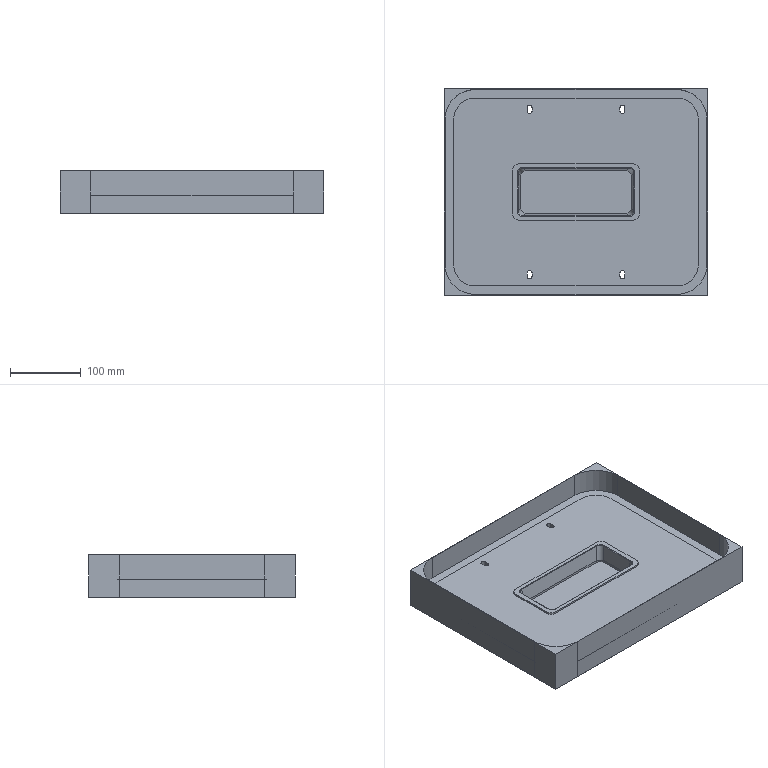NC program | NX | posted with a generic post | part box 371 x 291 x 60.5 mm
Lines 10591 to 11464 of 37416:
(CONTOUR_AREA , TOOL : R1.5)
N21174 M6
N21176 G53
N21178 G17 G0 G90 X-81.876 Y-39.38 S9000 M3 M8
N21180 G43 Z120.5 H0
N21182 Z31.3
N21184 G94 G1 Z28.3 F4500.
N21186 X-82.176 Y-39.321
N21188 X-82.462 Y-39.256
N21190 G2 X-85.472 Y-37.971 R8.221
N21192 G1 X-85.666 Y-37.853 Z28.298
N21194 X-85.775 Y-37.788 Z28.3
N21196 X-86.861 Y-36.859
N21198 X-87.633 Y-35.96
N21200 X-87.858 Y-35.66
N21202 X-87.873 Y-35.637
N21204 X-88.472 Y-34.658
N21206 X-88.565 Y-34.461
N21208 X-88.941 Y-33.562
N21210 X-89.074 Y-33.22
N21212 X-89.276 Y-32.367
N21214 X-89.374 Y-31.97
N21216 X-89.395 Y-31.764
N21218 X-89.486 Y-30.566
N21220 X-89.495 Y-29.967
N21222 Y30.264
N21224 X-89.486 Y30.554
N21226 Y30.566
N21228 X-89.396 Y31.75
N21230 X-89.374 Y31.97
N21232 X-89.205 Y32.663
N21234 X-89.074 Y33.22
N21236 X-88.941 Y33.56
N21238 X-88.566 Y34.458
N21240 X-88.474 Y34.656
N21242 X-87.874 Y35.636
N21244 X-87.858 Y35.66
N21246 X-87.635 Y35.958
N21248 X-86.861 Y36.859
N21250 X-85.775 Y37.788
N21252 X-84.575 Y38.51
N21254 X-83.375 Y39.013
N21256 X-83.075 Y39.102
N21258 X-82.176 Y39.319
N21260 X-81.876 Y39.38
N21262 X-80.676 Y39.483
N21264 X-80.376 Y39.496
N21266 X80.076
N21268 X80.376 Y39.492
N21270 X80.674 Y39.483
N21272 X81.855 Y39.382
N21274 X82.462 Y39.256
N21276 G2 X85.472 Y37.971 R8.221
N21278 G1 X85.666 Y37.853 Z28.298
N21280 X85.775 Y37.788 Z28.3
N21282 X86.861 Y36.859
N21284 X87.633 Y35.96
N21286 X87.873 Y35.637
N21288 X88.472 Y34.658
N21290 X88.565 Y34.461
N21292 X88.941 Y33.562
N21294 X89.074 Y33.22
N21296 X89.374 Y31.97
N21298 X89.395 Y31.764
N21300 X89.486 Y30.566
N21302 X89.494 Y30.266
N21304 X89.495 Y-29.967
N21306 X89.486 Y-30.554
N21308 X89.464 Y-30.855
N21310 X89.396 Y-31.75
N21312 X89.374 Y-31.97
N21314 X89.277 Y-32.364
N21316 X89.074 Y-33.22
N21318 X88.941 Y-33.56
N21320 X88.566 Y-34.458
N21322 X88.474 Y-34.656
N21324 X87.874 Y-35.637
N21326 X87.688 Y-35.886 Z28.299
N21328 X87.635 Y-35.958 Z28.3
N21330 X86.861 Y-36.859
N21332 X85.775 Y-37.788
N21334 X84.575 Y-38.51
N21336 X83.375 Y-39.013
N21338 X83.075 Y-39.102
N21340 X82.479 Y-39.251
N21342 X81.876 Y-39.38
N21344 X80.676 Y-39.483
N21346 X80.376 Y-39.492
N21348 X80.081 Y-39.496
N21350 X-80.372
N21352 X-80.674 Y-39.483
N21354 X-81.876 Y-39.38
N21356 X-81.84 Y-39.124
N21358 G2 X-86.722 Y-36.636 R8.88
N21360 X-88.876 Y-32.963 R8.803
N21362 G1 X-88.915 Y-32.804
N21364 X-89.02 Y-32.364
N21366 X-89.093 Y-32.064
N21368 X-89.139 Y-31.809
N21370 X-89.231 Y-30.566
N21372 X-89.245 Y-29.838
N21374 X-89.242 Y30.266
N21376 X-89.223 Y30.716
N21378 G2 X-83.375 Y38.74 R8.677
N21380 G1 X-83.244 Y38.788
N21382 G2 X-80.387 Y39.245 R9.754
N21384 G1 X80.366 Y39.246
N21386 G2 X86.722 Y36.636 R8.941
N21388 X88.875 Y32.963 R8.799
N21390 G1 X88.915 Y32.804
N21392 X88.949 Y32.663
N21394 X89.095 Y32.057
N21396 X89.136 Y31.807
N21398 X89.203 Y30.994
N21400 X89.238 Y30.43
N21402 X89.244 Y29.966
N21404 X89.243 Y-30.097
N21406 G2 X88.856 Y-33.034 R9.544
N21408 X88.174 Y-34.666 R7.729
N21410 G1 X87.874 Y-35.157
N21412 X87.747 Y-35.36
N21414 G2 X83.075 Y-38.837 R8.772
N21416 G1 X82.826 Y-38.906
N21418 X82.476 Y-38.994
N21420 X82.258 Y-39.043
N21422 G2 X80.387 Y-39.245 R9.523
N21424 G1 X-80.366
N21426 X-80.653 Y-39.233
N21428 X-81.755 Y-39.136
N21430 X-81.84 Y-39.124
N21432 X-81.798 Y-38.878
N21434 G2 X-88.981 Y-30.566 R8.474
N21436 G1 X-88.995 Y-29.887
N21438 X-88.99 Y30.349
N21440 G2 X-88.665 Y32.772 R9.062
N21442 X-82.788 Y38.657 R8.461
N21444 X-80.378 Y38.995 R9.822
N21446 G1 X-80.337
N21448 X80.375
N21450 G2 X85.596 Y37.279 R8.882
N21452 G1 X85.742 Y37.158
N21454 G2 X88.927 Y31.318 R8.336
N21456 G1 X88.986 Y30.478
N21458 X88.994 Y29.966
N21460 Y-30.046
N21462 G2 X88.665 Y-32.772 R9.424
N21464 X81.305 Y-38.927 R8.445
N21466 G1 X80.679 Y-38.981
N21468 X80.378 Y-38.995
N21470 X80.337
N21472 X-80.375
N21474 X-80.674 Y-38.981
N21476 X-81.528 Y-38.908
N21478 X-81.576 Y-38.903
N21480 X-81.798 Y-38.878
N21482 X-81.767 Y-38.629
N21484 G2 X-85.419 Y-37.102 R8.281
N21486 X-88.734 Y-30.526 R8.293
N21488 G1 X-88.74 Y-30.266
N21490 X-88.745 Y-29.937
N21492 X-88.743 Y30.297
N21494 G2 X-86.176 Y36.457 R8.436
N21496 X-80.076 Y38.745 R8.578
N21498 G1 X80.165
N21500 G2 X81.876 Y38.612 R13.516
N21502 X85.419 Y37.102 R8.783
N21504 X88.735 Y30.527 R8.297
N21506 G1 X88.744 Y30.236
N21508 X88.745 Y-29.966
N21510 G2 X88.297 Y-33.139 R9.253
N21512 G1 X88.094 Y-33.642
N21514 G2 X81.58 Y-38.653 R8.22
N21516 G1 X80.599 Y-38.733
N21518 X80.076 Y-38.745
N21520 X-80.165
N21522 G2 X-81.767 Y-38.629 R12.333
N21524 G1 X-81.733 Y-38.38
N21526 X-81.875 Y-38.36
N21528 G2 X-86.075 Y-36.212 R8.077
N21530 X-88.49 Y-30.285 R8.141
N21532 G1 X-88.495 Y-29.99
N21534 X-88.494 Y30.244
N21536 G2 X-86.016 Y36.259 R8.178
N21538 X-80.076 Y38.495 R8.262
N21540 G1 X80.214 Y38.494
N21542 G2 X84.275 Y37.522 R8.465
N21544 X88.482 Y30.576 R7.944
N21546 G1 X88.493 Y30.288
N21548 X88.495 Y-29.943
N21550 G2 X88.049 Y-33.088 R8.909
N21552 X80.548 Y-38.485 R8.037
N21554 G1 X80.076 Y-38.495
N21556 X-80.214 Y-38.494
N21558 X-80.676 Y-38.476
N21560 X-81.575 Y-38.401
N21562 X-81.733 Y-38.38
N21564 X-81.696 Y-38.13
N21566 G2 X-88.238 Y-30.33 R7.733
N21568 G1 X-88.243 Y-30.036
N21570 X-88.242 Y30.266
N21572 G2 X-88.119 Y31.819 R18.435
N21574 X-80.496 Y38.237 R7.781
N21576 G1 X-80.376 Y38.241
N21578 X-75.084 Y38.245
N21580 X80.263 Y38.244
N21582 G2 X84.894 Y36.859 R8.139
N21584 X88.242 Y30.266 R7.841
N21586 G1 X88.245 Y-29.896
N21588 G2 X88.119 Y-31.82 R16.142
N21590 X80.376 Y-38.241 R7.8
N21592 G1 X75.084 Y-38.245
N21594 X-80.263 Y-38.244
N21596 X-80.676 Y-38.226
N21598 X-81.576 Y-38.146
N21600 X-81.655 Y-38.136
N21602 X-81.696 Y-38.13
N21604 X-81.662 Y-37.881
N21606 G2 X-84.896 Y-36.559 R7.717
N21608 X-87.978 Y-30.566 R7.545
N21610 G1 X-87.993 Y-30.085
N21612 X-87.991 Y30.266
N21614 G2 X-84.875 Y36.557 R7.51
N21616 X-80.376 Y37.991 R7.778
N21618 G1 X80.312 Y37.993
N21620 G2 X84.896 Y36.559 R7.847
N21622 X87.979 Y30.566 R7.549
N21624 G1 X87.993 Y30.085
N21626 X87.992 Y-30.148
N21628 G2 X87.689 Y-32.549 R8.536
N21630 X80.444 Y-37.99 R7.546
N21632 G1 X80.376 Y-37.991
N21634 X-80.312 Y-37.993
N21636 X-80.676 Y-37.976
N21638 X-81.429 Y-37.91
N21640 X-81.576 Y-37.893
N21642 X-81.662 Y-37.881
N21644 X-81.623 Y-37.633
N21646 G2 X-87.719 Y-30.71 R7.214
N21648 G1 X-87.739 Y-30.266
N21650 X-87.745 Y-29.667
N21652 X-87.74 Y30.266
N21654 G2 X-87.444 Y32.494 R8.225
N21656 X-80.71 Y37.723 R7.267
N21658 G1 X-80.391 Y37.743
N21660 X80.362 Y37.744
N21662 G2 X85.798 Y35.41 R7.403
N21664 X87.728 Y30.566 R7.254
N21666 G1 X87.743 Y30.135
N21668 X87.742 Y-30.098
N21670 G2 X87.293 Y-32.961 R8.388
N21672 X80.71 Y-37.723 R7.266
N21674 G1 X80.391 Y-37.743
N21676 X-80.362 Y-37.744
N21678 X-80.647 Y-37.728
N21680 X-81.472 Y-37.654
N21682 X-81.576 Y-37.64
N21684 X-81.623 Y-37.633
N21686 X-81.576 Y-37.388
N21688 G2 X-87.444 Y-31.035 R6.93
N21690 G1 X-87.482 Y-30.474
N21692 X-87.495 Y-29.887
N21694 X-87.491 Y30.266
N21696 G2 X-87.2 Y32.438 R8.021
N21698 X-80.678 Y37.475 R7.013
N21700 G1 X-80.378 Y37.493
N21702 X80.375
N21704 G2 X82.576 Y37.158 R8.238
N21706 X87.465 Y30.756 R6.936
N21708 G1 X87.49 Y30.266
N21710 X87.493 Y-30.047
N21712 G2 X87.2 Y-32.437 R8.292
N21714 X80.678 Y-37.475 R7.014
N21716 G1 X80.378 Y-37.493
N21718 X-80.375
N21720 G2 X-81.576 Y-37.388 R20.153
N21722 G1 X-81.558 Y-37.14
N21724 G2 X-87.231 Y-30.522 R6.727
N21726 G1 X-87.24 Y-30.232
N21728 X-87.245 Y-29.937
N21730 X-87.241 Y30.299
N21732 G2 X-86.958 Y32.38 R7.788
N21734 X-80.376 Y37.239 R6.804
N21736 G1 X-80.292 Y37.242
N21738 X80.162 Y37.244
N21740 G2 X83.405 Y36.559 R7.492
N21742 X87.231 Y30.522 R6.711
N21744 G1 X87.242 Y30.266
N21746 Y30.234
N21748 X87.244 Y-29.997
N21750 G2 X86.974 Y-32.319 R8.104
N21752 X80.376 Y-37.239 R6.81
N21754 G1 X80.292 Y-37.242
N21756 X-80.162 Y-37.244
N21758 G2 X-81.558 Y-37.14 R13.174
N21760 G1 X-81.526 Y-36.89
N21762 G2 X-85.175 Y-34.983 R6.642
N21764 X-86.989 Y-30.283 R6.6
N21766 G1 X-86.994 Y-29.989
N21768 X-86.993 Y30.245
N21770 G2 X-86.712 Y32.326 R8.362
N21772 X-80.554 Y36.981 R6.552
N21774 G1 X-80.076 Y36.994
N21776 X80.211 Y36.993
N21778 G2 X83.451 Y36.259 R7.021
N21780 X86.992 Y30.287 R6.567
N21782 G1 X86.995 Y-29.944
N21784 G2 X86.891 Y-31.548 R15.293
N21786 X80.554 Y-36.981 R6.538
N21788 G1 X80.076 Y-36.994
N21790 X-80.211 Y-36.993
N21792 X-80.676 Y-36.971
N21794 X-81.332 Y-36.914
N21796 X-81.526 Y-36.89
N21798 X-81.491 Y-36.639
N21800 G2 X-86.724 Y-30.618 R6.204
N21802 G1 X-86.743 Y-30.035
N21804 X-86.74 Y30.266
N21806 G2 X-82.476 Y36.39 R6.285
N21808 X-80.376 Y36.738 R6.535
N21810 G1 X-79.891 Y36.744
N21812 X80.26 Y36.742
N21814 G2 X84.323 Y35.409 R6.542
N21816 X86.724 Y30.618 R6.252
N21818 G1 X86.738 Y30.33
N21820 X86.74 Y30.266
N21822 X86.744 Y-29.897
N21824 G2 X86.519 Y-32.064 R7.88
N21826 X80.976 Y-36.697 R6.252
N21828 G1 X80.376 Y-36.738
N21830 X79.891 Y-36.744
N21832 X-80.26 Y-36.742
N21834 X-80.676 Y-36.721
N21836 X-81.373 Y-36.655
N21838 X-81.491 Y-36.639
N21840 X-81.45 Y-36.39
N21842 G2 X-86.475 Y-30.566 R5.969
N21844 G1 X-86.493 Y-29.966
N21846 X-86.492 Y30.149
N21848 G2 X-86.324 Y31.815 R8.539
N21850 X-80.976 Y36.446 R6.002
N21852 G1 X-80.376 Y36.489
N21854 X-80.142 Y36.493
N21856 X-79.841 Y36.494
N21858 X80.076 Y36.495
N21860 G2 X82.379 Y36.163 R7.225
N21862 X86.475 Y30.566 R5.962
N21864 G1 X86.492 Y30.084
N21866 X86.493 Y-29.966
N21868 G2 X86.323 Y-31.816 R8.65
N21870 X80.976 Y-36.446 R6.
N21872 G1 X80.376 Y-36.489
N21874 X80.142 Y-36.493
N21876 X79.841 Y-36.494
N21878 X-80.076 Y-36.495
N21880 G2 X-81.45 Y-36.39 R9.833
N21882 G1 X-81.414 Y-36.142
N21884 G2 X-86.224 Y-30.566 R5.692
N21886 G1 X-86.243 Y-29.966
N21888 X-86.242 Y30.099
N21890 G2 X-86.08 Y31.761 R8.098
N21892 X-81.047 Y36.189 R5.758
N21894 G1 X-80.376 Y36.24
N21896 X80.063 Y36.246
N21898 G2 X83.038 Y35.622 R6.562
N21900 X86.224 Y30.566 R5.735
N21902 G1 X86.241 Y30.133
N21904 Y-30.099
N21906 G2 X86.079 Y-31.759 R7.93
N21908 X81.047 Y-36.189 R5.755
N21910 G1 X80.376 Y-36.24
N21912 X-80.063 Y-36.246
N21914 G2 X-81.414 Y-36.142 R11.267
N21916 G1 X-81.374 Y-35.895
N21918 G2 X-85.973 Y-30.566 R5.472
N21920 G1 X-85.99 Y-30.181
N21922 X-85.995 Y-28.744
N21924 X-85.989 Y30.266
N21926 G2 X-85.635 Y32.364 R5.858
N21928 X-80.678 Y35.97 R5.547
N21930 G1 X-80.378 Y35.991
N21932 X80.075 Y35.995
N21934 G2 X83.075 Y35.322 R6.189
N21936 X85.98 Y30.471 R5.496
N21938 G1 X85.988 Y30.266
N21940 X85.991 Y30.182
N21942 X85.992 Y-30.049
N21944 G2 X85.731 Y-32.108 R7.171
N21946 X80.678 Y-35.97 R5.542
N21948 G1 X80.378 Y-35.991
N21950 X-80.075 Y-35.995
N21952 G2 X-81.374 Y-35.895 R10.8
N21954 G1 X-81.33 Y-35.65
N21956 G2 X-85.727 Y-30.518 R5.238
N21958 G1 X-85.739 Y-30.23
N21960 X-85.744 Y-29.936
N21962 X-85.739 Y30.302
N21964 G2 X-85.175 Y32.802 R5.596
N21966 X-80.296 Y35.74 R5.36
N21968 G1 X80.159 Y35.743
N21970 G2 X83.029 Y35.061 R5.767
N21972 X85.727 Y30.518 R5.223
N21974 G1 X85.74 Y30.266
N21976 X85.741 Y30.232
N21978 X85.743 Y-29.998
N21980 G2 X85.296 Y-32.542 R6.203
N21982 X80.296 Y-35.74 R5.34
N21984 G1 X-80.16 Y-35.743
N21986 G2 X-81.33 Y-35.65 R10.7
N21988 G1 X-81.276 Y-35.406
N21990 G2 X-85.474 Y-30.566 R4.977
N21992 G1 X-85.488 Y-30.282
N21994 X-85.494 Y-29.988
N21996 X-85.492 Y30.247
N21998 G2 X-85.043 Y32.495 R5.441
N22000 X-80.561 Y35.476 R5.077
N22002 G1 X-80.076 Y35.493
N22004 X80.076 Y35.494
N22006 G2 X82.256 Y35.141 R5.591
N22008 X85.474 Y30.566 R4.961
N22010 G1 X85.49 Y30.284
N22012 X85.494 Y-29.945
N22014 G2 X85.346 Y-31.594 R8.901
N22016 X80.676 Y-35.467 R5.035
N22018 G1 X80.246 Y-35.491
N22020 X-80.076 Y-35.494
N22022 X-80.495 Y-35.479
N22024 X-81.048 Y-35.432
N22026 X-81.276 Y-35.406
N22028 X-81.243 Y-35.154
N22030 G2 X-85.22 Y-30.614 R4.701
N22032 G1 X-85.235 Y-30.326
N22034 X-85.244 Y-29.736
N22036 X-85.238 Y30.266
N22038 G2 X-85.104 Y31.536 R8.022
N22040 X-80.676 Y35.216 R4.796
N22042 G1 X-80.195 Y35.241
N22044 X80.076 Y35.243
N22046 G2 X82.271 Y34.865 R5.459
N22048 X85.22 Y30.614 R4.704
N22050 G1 X85.237 Y30.328
N22052 X85.243 Y28.816
N22054 Y-29.966
N22056 G2 X85.102 Y-31.537 R8.119
N22058 X80.676 Y-35.216 R4.792
N22060 G1 X80.195 Y-35.241
N22062 X-80.076 Y-35.243
N22064 X-80.541 Y-35.225
N22066 X-81.09 Y-35.174
N22068 X-81.243 Y-35.154
N22070 X-81.203 Y-34.904
N22072 G2 X-84.943 Y-30.934 R4.436
N22074 G1 X-84.981 Y-30.372
N22076 X-84.994 Y-29.786
N22078 X-84.99 Y30.151
N22080 G2 X-84.741 Y31.898 R5.317
N22082 X-80.376 Y34.985 R4.578
N22084 G1 X-79.843 Y34.994
N22086 X80.076
N22088 G2 X82.481 Y34.5 R5.375
N22090 X84.943 Y30.934 R4.427
N22092 G1 X84.982 Y30.373
N22094 X84.992 Y29.784
N22096 Y-29.966
N22098 X84.977 Y-30.463
N22100 G2 X80.376 Y-34.985 R4.558
N22102 G1 X79.843 Y-34.994
N22104 X-80.076
N22106 X-80.304 Y-34.989
N22108 X-80.376 Y-34.985
N22110 X-80.863 Y-34.947
N22112 X-81.203 Y-34.904
N22114 X-81.172 Y-34.657
N22116 G2 X-84.696 Y-30.865 R4.176
N22118 G1 X-84.728 Y-30.419
N22120 X-84.744 Y-29.835
N22122 X-84.74 Y30.101
N22124 G2 X-84.402 Y32.064 R4.904
N22126 X-80.376 Y34.736 R4.36
N22128 G1 X-80.076 Y34.744
N22130 X-76.494
N22132 X80.06 Y34.745
N22134 G2 X82.476 Y34.221 R5.07
N22136 X84.696 Y30.865 R4.148
N22138 G1 X84.729 Y30.42
N22140 X84.742 Y29.966
N22142 Y-29.966
N22144 G2 X84.494 Y-31.845 R6.157
N22146 X80.376 Y-34.736 R4.377
N22148 G1 X80.076 Y-34.744
N22150 X76.494
N22152 X-80.06 Y-34.745
N22154 G2 X-81.172 Y-34.657 R7.776
N22156 G1 X-81.134 Y-34.409
N22158 G2 X-84.444 Y-30.865 R3.913
N22160 G1 X-84.475 Y-30.466
N22162 X-84.493 Y-29.966
N22164 X-84.491 Y30.051
N22166 G2 X-84.258 Y31.764 R5.752
N22168 X-80.376 Y34.487 R4.117
N22170 G1 X-80.078 Y34.494
N22172 X-76.779
N22174 X-74.68 Y34.495 Z28.282
N22176 X75.278 Y34.496 Z28.284
N22178 X76.741 Y34.495 Z28.3
N22180 X80.074
N22182 G2 X82.176 Y34.086 R4.762
N22184 X84.476 Y30.467 R3.972
N22186 G1 X84.486 Y30.266
N22188 X84.489 Y30.18
N22190 X84.491 Y-30.05
N22192 G2 X84.259 Y-31.764 R5.341
N22194 X80.376 Y-34.487 R4.118
N22196 G1 X80.078 Y-34.494
N22198 X76.779
N22200 X74.68 Y-34.495 Z28.282
N22202 X-75.278 Y-34.496 Z28.284
N22204 X-76.741 Y-34.495 Z28.3
N22206 X-80.074
N22208 G2 X-81.134 Y-34.409 R8.021
N22210 G1 X-81.114 Y-34.162
N22212 G2 X-84.2 Y-30.791 R3.703
N22214 G1 X-84.236 Y-30.266
N22216 X-84.244 Y-29.667
N22218 X-84.241 Y30.
N22220 G2 X-83.99 Y31.762 R5.216
N22222 X-80.376 Y34.233 R3.857
N22224 G1 X-79.776 Y34.244
N22226 X-77.212 Z28.297
N22228 X-75.878 Y34.247 Z28.255
N22230 X-74.678 Y34.248 Z28.242
N22232 X75.278 Y34.249 Z28.245
N22234 X76.477 Y34.247 Z28.271
N22236 X77.21 Y34.245 Z28.297
N22238 X79.86 Z28.3
N22240 G2 X81.576 Y34.048 R5.447
N22242 X84.2 Y30.791 R3.648
N22244 G1 X84.239 Y30.23
N22246 X84.243 Y-29.998
N22248 G2 X83.99 Y-31.762 R5.276
N22250 X80.376 Y-34.233 R3.857
N22252 G1 X79.776 Y-34.244
N22254 X77.212 Z28.297
N22256 X75.878 Y-34.247 Z28.255
N22258 X74.678 Y-34.248 Z28.242
N22260 X-75.278 Y-34.249 Z28.245
N22262 X-76.477 Y-34.247 Z28.271
N22264 X-77.21 Y-34.245 Z28.297
N22266 X-79.86 Z28.3
N22268 G2 X-81.114 Y-34.162 R8.529
N22270 G1 X-81.068 Y-33.913
N22272 G2 X-83.975 Y-30.476 R3.466
N22274 G1 X-83.986 Y-30.279
N22276 X-83.994 Y-29.987
N22278 X-83.989 Y30.25
N22280 G2 X-82.551 Y33.263 R3.632
N22282 X-80.376 Y33.982 R3.663
N22284 G1 X-79.945 Y33.993
N22286 X-79.776 Y33.994
N22288 X-79.177
N22290 X-78.145
N22292 X-77.977 Z28.294
N22294 X-77.845
N22296 X-75.878 Y34.001 Z28.208
N22298 X-75.136 Y34.004 Z28.191
N22300 X-73.511 Z28.186
N22302 X74.978 Y34.005 Z28.188
N22304 X75.737 Y34.003 Z28.205
N22306 X76.777 Y33.999 Z28.245
N22308 X77.543 Y33.996 Z28.282
N22310 X78.144 Y33.995 Z28.3
N22312 X78.443
N22314 X79.477
N22316 G2 X81.325 Y33.862 R7.867
N22318 X83.946 Y30.836 R3.438
N22320 G1 X83.987 Y30.281
N22322 X83.992 Y29.986
N22324 X83.994 Y-29.945
N22326 G2 X83.675 Y-31.856 R4.506
N22328 X80.376 Y-33.982 R3.596
N22330 G1 X79.945 Y-33.993
N22332 X79.776 Y-33.994
N22334 X79.177
N22336 X78.145
N22338 X77.977 Z28.294
N22340 X77.845
N22342 X75.878 Y-34.001 Z28.208
N22344 X75.136 Y-34.004 Z28.191
N22346 X73.511 Z28.186
N22348 X-74.978 Y-34.005 Z28.188
N22350 X-75.737 Y-34.003 Z28.205
N22352 X-76.777 Y-33.999 Z28.245
N22354 X-77.543 Y-33.996 Z28.282
N22356 X-78.144 Y-33.995 Z28.3
N22358 X-78.443
N22360 X-79.477
N22362 X-80.204 Y-33.989
N22364 X-80.676 Y-33.959
N22366 X-81.033 Y-33.919
N22368 X-81.068 Y-33.913
N22370 X-81.028 Y-33.662
N22372 G2 X-83.715 Y-30.61 R3.18
N22374 G1 X-83.733 Y-30.325
N22376 X-83.744 Y-29.735
N22378 X-83.738 Y30.203
N22380 G2 X-83.492 Y31.647 R3.994
N22382 X-80.376 Y33.731 R3.332
N22384 G1 X-79.895 Y33.743
N22386 X-79.295 Y33.744
N22388 X-78.513 Z28.299
N22390 X-77.793 Y33.746 Z28.262
N22392 X-76.888 Y33.751 Z28.205
N22394 X-76.777 Y33.753 Z28.193
N22396 X-76.283 Y33.757 Z28.163
N22398 X-76.178 Y33.76 Z28.152
N22400 X-75.578 Y33.765 Z28.121
N22402 X-74.678 Y33.769 Z28.103
N22404 X74.978 Z28.107
N22406 X75.578 Y33.766 Z28.121
N22408 X76.178 Y33.761 Z28.153
N22410 X76.585 Y33.755 Z28.185
N22412 X76.777 Y33.754 Z28.194
N22414 X76.887 Y33.752 Z28.205
N22416 X78.093 Y33.746 Z28.281
N22418 X78.277 Z28.287
N22420 X78.511 Y33.745 Z28.299
N22422 X78.877 Z28.3
N22424 X79.659
N22426 G2 X81.318 Y33.604 R6.883
N22428 X83.715 Y30.61 R3.193
N22430 G1 X83.734 Y30.326
N22432 X83.741 Y30.032
N22434 X83.742 Y29.734
N22436 Y-29.966
N22438 X83.722 Y-30.519
N22440 G2 X80.376 Y-33.731 R3.322
N22442 G1 X79.895 Y-33.743
N22444 X79.295 Y-33.744
N22446 X78.513 Z28.299
N22448 X77.793 Y-33.746 Z28.262
N22450 X76.888 Y-33.751 Z28.205
N22452 X76.777 Y-33.753 Z28.193
N22454 X76.283 Y-33.757 Z28.163
N22456 X76.178 Y-33.76 Z28.152
N22458 X75.578 Y-33.765 Z28.121
N22460 X74.678 Y-33.769 Z28.103
N22462 X-74.978 Z28.107
N22464 X-75.578 Y-33.766 Z28.121
N22466 X-76.178 Y-33.761 Z28.153
N22468 X-76.585 Y-33.755 Z28.185
N22470 X-76.777 Y-33.754 Z28.194
N22472 X-76.887 Y-33.752 Z28.205
N22474 X-78.093 Y-33.746 Z28.281
N22476 X-78.277 Z28.287
N22478 X-78.511 Y-33.745 Z28.299
N22480 X-78.877 Z28.3
N22482 X-79.659
N22484 X-80.251 Y-33.737
N22486 X-80.676 Y-33.707
N22488 X-81.028 Y-33.662
N22490 X-80.976 Y-33.416
N22492 G2 X-83.438 Y-30.865 R2.923
N22494 G1 X-83.478 Y-30.369
N22496 X-83.492 Y-29.966
N22498 X-83.488 Y30.153
N22500 G2 X-83.394 Y31.154 R6.014
N22502 X-80.376 Y33.481 R3.105
N22504 G1 X-80.148 Y33.491
N22506 X-80.076 Y33.492
N22508 X-79.845 Y33.494
N22510 X-79.245
N22512 X-78.877 Z28.294
N22514 X-78.645 Z28.286
N22516 X-78.577 Y33.495 Z28.28
N22518 X-77.499 Y33.501 Z28.199
N22520 X-76.477 Y33.52 Z28.09
N22522 X-76.213 Y33.527 Z28.062
N22524 X-76.178 Y33.528 Z28.058
N22526 X-75.578 Y33.539 Z28.015
N22528 X-75.278 Y33.542 Z28.003
N22530 X-74.997 Y33.543 Z27.996
N22532 X-74.678 Y33.545 Z27.991
N22534 X74.662 Y33.546
N22536 X74.978 Y33.545 Z27.996
N22538 X75.278 Y33.543 Z28.003
N22540 X75.578 Y33.54 Z28.015
N22542 X76.212 Y33.528 Z28.063
N22544 X77.077 Y33.51 Z28.153
N22546 X77.497 Y33.502 Z28.199
N22548 X78.644 Y33.495 Z28.286
N22550 X78.877 Z28.294
N22552 X78.944 Z28.299
N22554 X79.709 Z28.3
N22556 G2 X81.57 Y33.257 R5.443
N22558 X83.479 Y30.369 R2.994
N22560 G1 X83.491 Y29.966
N22562 X83.492 Y-29.966
N22564 X83.473 Y-30.468
N22566 G2 X80.376 Y-33.481 R3.074
N22568 G1 X80.148 Y-33.491
N22570 X80.076 Y-33.492
N22572 X79.845 Y-33.494
N22574 X79.245
N22576 X78.877 Z28.294
N22578 X78.645 Z28.286
N22580 X78.577 Y-33.495 Z28.28
N22582 X77.499 Y-33.501 Z28.199
N22584 X76.477 Y-33.52 Z28.09
N22586 X76.213 Y-33.526 Z28.062
N22588 X76.169 Y-33.528 Z28.057
N22590 X75.9 Y-33.532 Z28.038
N22592 X75.578 Y-33.539 Z28.015
N22594 X75.278 Y-33.542 Z28.003
N22596 X74.997 Y-33.543 Z27.996
N22598 X74.678 Y-33.545 Z27.991
N22600 X-74.662 Y-33.546
N22602 X-74.978 Y-33.545 Z27.996
N22604 X-75.278 Y-33.543 Z28.003
N22606 X-75.578 Y-33.54 Z28.015
N22608 X-76.212 Y-33.528 Z28.063
N22610 X-77.077 Y-33.51 Z28.153
N22612 X-77.497 Y-33.502 Z28.199
N22614 X-78.644 Y-33.495 Z28.286
N22616 X-78.877 Z28.294
N22618 X-78.944 Z28.299
N22620 X-79.709 Z28.3
N22622 G2 X-80.976 Y-33.416 R7.385
N22624 G1 X-80.932 Y-33.169
N22626 G2 X-83.213 Y-30.566 R2.691
N22628 G1 X-83.238 Y-30.129
N22630 X-83.244 Y-29.667
N22632 X-83.239 Y30.103
N22634 G2 X-83.023 Y31.465 R3.669
N22636 X-80.376 Y33.232 R2.879
N22638 G1 X-80.096 Y33.243
N22640 X-79.795 Y33.244
N22642 X-79.477
N22644 X-79.214 Z28.296
N22646 X-78.277 Y33.249 Z28.219
N22648 X-77.988 Y33.252 Z28.191
N22650 X-77.977 Z28.189
N22652 X-77.377 Y33.266 Z28.104
N22654 X-76.75 Y33.29 Z28.006
N22656 X-76.131 Y33.309 Z27.934
N22658 X-75.518 Y33.322 Z27.888
N22660 X-75.283 Y33.326 Z27.876
N22662 X-74.982 Y33.328 Z27.868
N22664 X-74.682 Y33.33 Z27.863
N22666 X74.674 Y33.331 Z27.864
N22668 X75.278 Y33.327 Z27.877
N22670 X75.513 Y33.323 Z27.888
N22672 X75.578 Z27.891
N22674 X76.178 Y33.31 Z27.938
N22676 X76.777 Y33.291 Z28.009
N22678 X77.681 Y33.259 Z28.151
N22680 X77.977 Y33.253 Z28.19
N22682 X77.987 Z28.191
N22684 X78.893 Y33.246 Z28.273
N22686 X79.212 Y33.245 Z28.296
N22688 X79.477 Z28.3
N22690 X79.776
N22692 X80.076 Y33.239
N22694 G2 X82.176 Y32.634 R3.4
N22696 X83.214 Y30.566 R2.743
N22698 G1 X83.238 Y30.129
N22700 X83.242 Y26.913
N22702 X83.241 Y-29.966
N22704 G2 X82.987 Y-31.553 R3.803
N22706 X80.376 Y-33.232 R2.888
N22708 G1 X80.096 Y-33.243
N22710 X79.795 Y-33.244
N22712 X79.477
N22714 X79.214 Z28.296
N22716 X78.277 Y-33.249 Z28.219
N22718 X77.988 Y-33.252 Z28.191
N22720 X77.977 Z28.189
N22722 X77.377 Y-33.266 Z28.104
N22724 X76.75 Y-33.29 Z28.006
N22726 X76.116 Y-33.311 Z27.93
N22728 X75.518 Y-33.322 Z27.888
N22730 X75.283 Y-33.326 Z27.876
N22732 X74.982 Y-33.328 Z27.868
N22734 X74.682 Y-33.33 Z27.863
N22736 X-74.674 Y-33.331 Z27.864
N22738 X-75.278 Y-33.327 Z27.877
N22740 X-75.513 Y-33.323 Z27.888
N22742 X-75.578 Z27.891
N22744 X-76.178 Y-33.31 Z27.938
N22746 X-76.777 Y-33.291 Z28.009
N22748 X-77.681 Y-33.259 Z28.151
N22750 X-77.977 Y-33.253 Z28.19
N22752 X-77.987 Z28.191
N22754 X-79.177 Y-33.245 Z28.293
N22756 X-79.776 Z28.3
N22758 X-80.076 Y-33.239
N22760 G2 X-80.932 Y-33.169 R5.319
N22762 G1 X-80.896 Y-32.922
N22764 G2 X-82.962 Y-30.566 R2.441
N22766 G1 X-82.971 Y-30.461
N22768 X-82.992 Y-29.966
N22770 X-82.989 Y30.052
N22772 G2 X-82.731 Y31.51 R3.32
N22774 X-80.379 Y32.982 R2.64
N22776 G1 X-80.078 Y32.993
N22778 X-79.715 Y32.994
N22780 X-79.477 Z28.291
N22782 X-78.539 Y33.001 Z28.202
N22784 X-78.279 Y33.006 Z28.162
N22786 X-78.234 Z28.157
N22788 X-77.979 Y33.016 Z28.108
N22790 X-77.923 Y33.017 Z28.101
N22792 X-77.293 Y33.047 Z27.977
N22794 X-76.98 Y33.06 Z27.925
N22796 X-76.777 Y33.071 Z27.889
N22798 X-76.178 Y33.099 Z27.803
N22800 X-76.039 Y33.102 Z27.791
N22802 X-75.878 Y33.111 Z27.77
N22804 X-75.727 Y33.113 Z27.759
N22806 X-75.578 Y33.121 Z27.743
N22808 X-75.418 Y33.122 Z27.736
N22810 X-75.278 Y33.128 Z27.725
N22812 X-74.508 Y33.133 Z27.709
N22814 X74.808 Y33.132 Z27.714
N22816 X75.278 Y33.129 Z27.726
N22818 X75.417 Y33.123 Z27.736
N22820 X75.578 Y33.122 Z27.744
N22822 X75.726 Y33.114 Z27.76
N22824 X75.878 Y33.112 Z27.771
N22826 X76.178 Y33.095 Z27.81
N22828 X76.219 Y33.092 Z27.817
N22830 X76.477 Y33.085 Z27.846
N22832 X76.665 Y33.075 Z27.876
N22834 X76.777 Y33.072 Z27.89
N22836 X77.377 Y33.045 Z27.991
N22838 X77.921 Y33.018 Z28.101
N22840 X78.277 Y33.007 Z28.162
N22842 X78.536 Y33.002 Z28.202
N22844 X78.577 Y33.001 Z28.206
N22846 X79.477 Y32.995 Z28.291
N22848 X79.713 Z28.3
N22850 X80.043 Y32.994
N22852 X80.076
N22854 G2 X81.972 Y32.473 R3.172
N22856 X82.971 Y30.461 R2.52
N22858 G1 X82.983 Y30.266
N22860 X82.987 Y30.177
N22862 X82.992 Y29.667
N22864 X82.99 Y-30.051
N22866 G2 X82.731 Y-31.509 R3.357
N22868 X80.379 Y-32.982 R2.64
N22870 G1 X80.078 Y-32.993
N22872 X79.715 Y-32.994
N22874 X79.477 Z28.291
N22876 X78.539 Y-33.001 Z28.202
N22878 X78.279 Y-33.006 Z28.162
N22880 X78.234 Z28.157
N22882 X77.979 Y-33.016 Z28.108
N22884 X77.923 Y-33.017 Z28.101
N22886 X77.293 Y-33.047 Z27.977
N22888 X76.98 Y-33.06 Z27.925
N22890 X76.777 Y-33.071 Z27.889
N22892 X75.987 Y-33.108 Z27.778
N22894 X75.727 Y-33.113 Z27.759
N22896 X75.578 Y-33.121 Z27.743
N22898 X75.418 Y-33.122 Z27.736
N22900 X75.278 Y-33.128 Z27.725
N22902 X74.678 Y-33.133 Z27.71
N22904 X-74.808 Y-33.132 Z27.714
N22906 X-75.278 Y-33.129 Z27.726
N22908 X-75.417 Y-33.123 Z27.736
N22910 X-75.578 Y-33.122 Z27.744
N22912 X-75.726 Y-33.114 Z27.76
N22914 X-75.878 Y-33.112 Z27.771